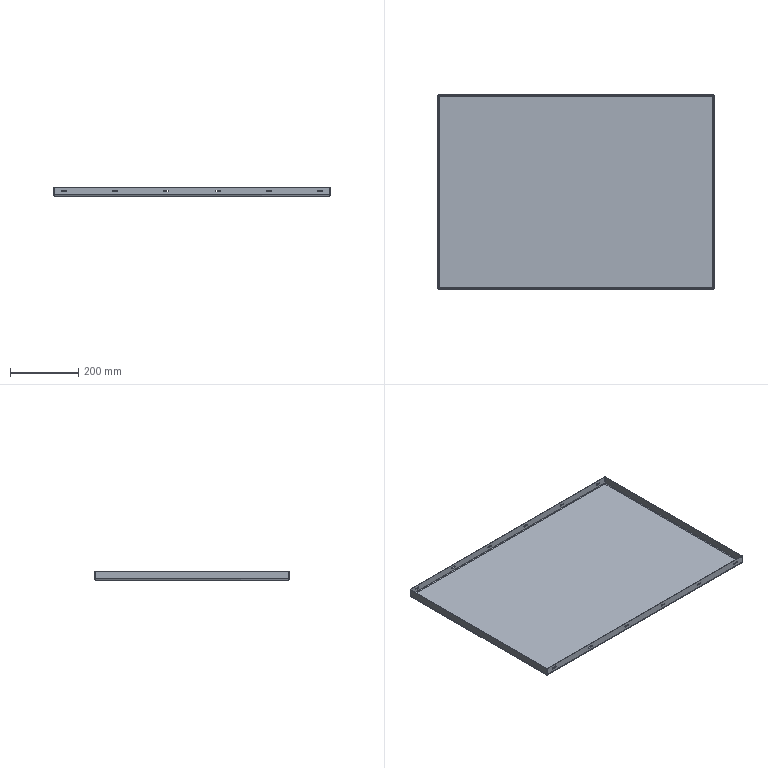Part | SolidWorks | features EdgeFlange 1, FlatPattern 1, ICE 1, SMBaseFlange 1, SheetMetal 1 | 1 solid | 86 faces | box 810 x 570 x 25 mm | volume 1040756 mm3 | plane 46 | cylinder 32 | spline 8 | commonest cylinder face diameters 4.5 x24 4 x4 8 x4